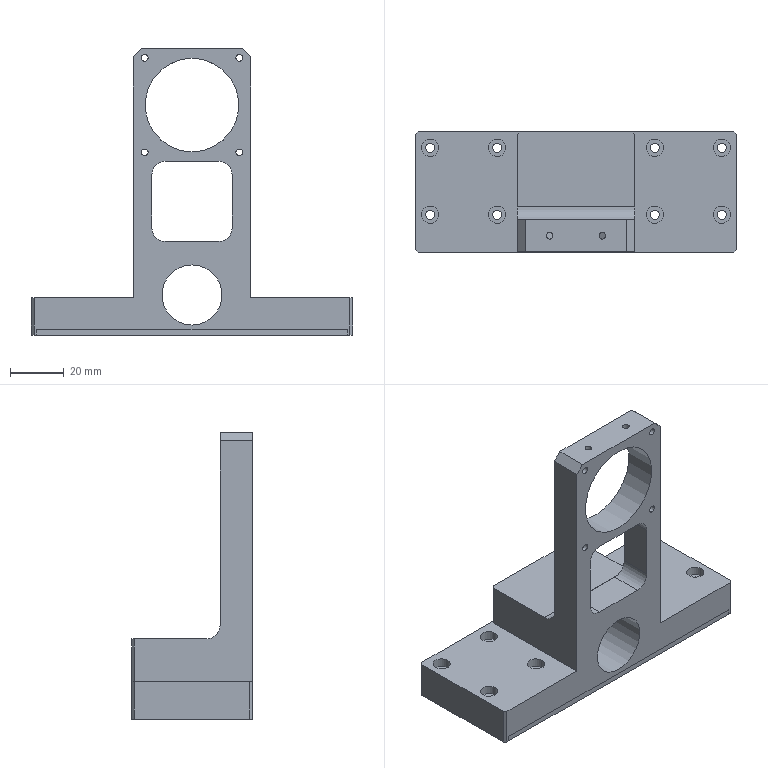Part | 2 solids | 150 faces | box 120 x 45 x 107 mm | volume 200954 mm3 | cylinder 70 | plane 68 | cone 12 | commonest cylinder face diameters 2.5 x16 3.4 x16 6.5 x16 10 x10 3.3 x8 22.5 x2